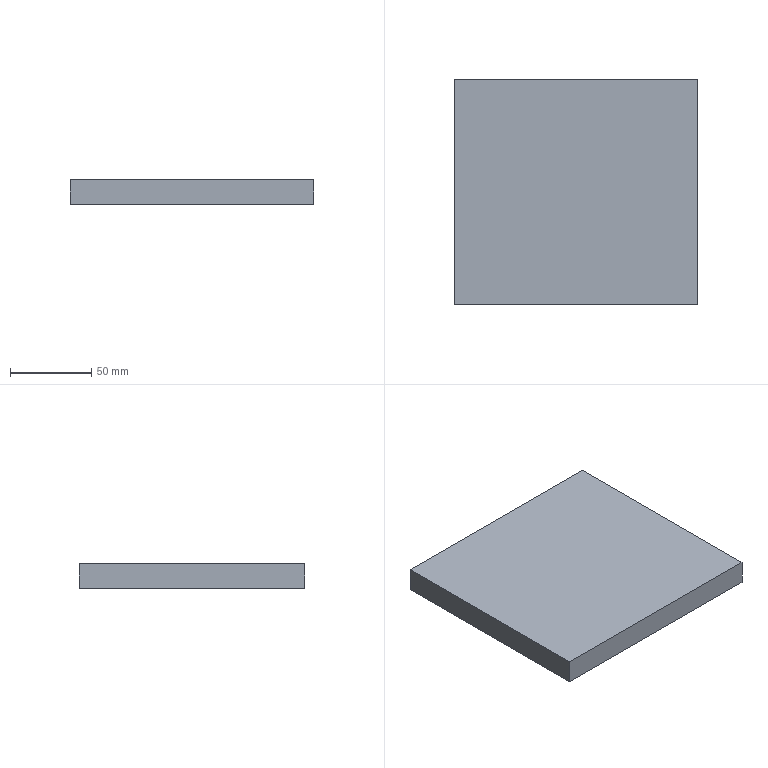Part | STEP file | PN_0004 | 1 solid | 6 faces | box 150 x 139 x 15 mm | volume 312750 mm3 | plane 6
STEP:
#1=CARTESIAN_POINT('',(0.,0.,0.));
#2=DIRECTION('',(0.,0.,1.));
#3=DIRECTION('',(1.,0.,0.));
#4=AXIS2_PLACEMENT_3D('',#1,#2,#3);
#5=CARTESIAN_POINT('',(75.,-69.5,0.));
#6=VERTEX_POINT('',#5);
#7=CARTESIAN_POINT('',(75.,69.5,0.));
#8=VERTEX_POINT('',#7);
#9=CARTESIAN_POINT('',(75.,69.5,0.));
#10=DIRECTION('',(0.,1.,0.));
#11=VECTOR('',#10,1.);
#12=LINE('',#9,#11);
#13=CARTESIAN_POINT('',(75.,69.5,15.));
#14=DIRECTION('',(-1.,0.,0.));
#15=DIRECTION('',(0.,-1.,0.));
#16=AXIS2_PLACEMENT_3D('',#13,#14,#15);
#17=PLANE('',#16);
#18=CARTESIAN_POINT('',(0.,-15.));
#19=DIRECTION('',(-1.,0.));
#20=VECTOR('',#19,1.);
#21=LINE('',#18,#20);
#22=(GEOMETRIC_REPRESENTATION_CONTEXT(2)PARAMETRIC_REPRESENTATION_CONTEXT()REPRESENTATION_CONTEXT('',''));
#23=DEFINITIONAL_REPRESENTATION('',(#21),#22);
#24=PCURVE('',#17,#23);
#25=CARTESIAN_POINT('',(75.,-69.5,0.));
#26=DIRECTION('',(0.,0.,1.));
#27=DIRECTION('',(1.,0.,0.));
#28=AXIS2_PLACEMENT_3D('',#25,#26,#27);
#29=PLANE('',#28);
#30=CARTESIAN_POINT('',(0.,139.));
#31=DIRECTION('',(0.,1.));
#32=VECTOR('',#31,1.);
#33=LINE('',#30,#32);
#34=(GEOMETRIC_REPRESENTATION_CONTEXT(2)PARAMETRIC_REPRESENTATION_CONTEXT()REPRESENTATION_CONTEXT('',''));
#35=DEFINITIONAL_REPRESENTATION('',(#33),#34);
#36=PCURVE('',#29,#35);
#37=SURFACE_CURVE('',#12,(#24,#36),.PCURVE_S1.);
#38=EDGE_CURVE('',#6,#8,#37,.T.);
#39=ORIENTED_EDGE('',*,*,#38,.T.);
#40=CARTESIAN_POINT('',(75.,69.5,15.));
#41=VERTEX_POINT('',#40);
#42=CARTESIAN_POINT('',(75.,69.5,15.));
#43=DIRECTION('',(0.,0.,-1.));
#44=VECTOR('',#43,1.);
#45=LINE('',#42,#44);
#46=CARTESIAN_POINT('',(0.,0.));
#47=DIRECTION('',(0.,-1.));
#48=VECTOR('',#47,1.);
#49=LINE('',#46,#48);
#50=(GEOMETRIC_REPRESENTATION_CONTEXT(2)PARAMETRIC_REPRESENTATION_CONTEXT()REPRESENTATION_CONTEXT('',''));
#51=DEFINITIONAL_REPRESENTATION('',(#49),#50);
#52=PCURVE('',#17,#51);
#53=CARTESIAN_POINT('',(-75.,69.5,15.));
#54=DIRECTION('',(0.,-1.,0.));
#55=DIRECTION('',(0.,0.,-1.));
#56=AXIS2_PLACEMENT_3D('',#53,#54,#55);
#57=PLANE('',#56);
#58=CARTESIAN_POINT('',(0.,150.));
#59=DIRECTION('',(1.,0.));
#60=VECTOR('',#59,1.);
#61=LINE('',#58,#60);
#62=(GEOMETRIC_REPRESENTATION_CONTEXT(2)PARAMETRIC_REPRESENTATION_CONTEXT()REPRESENTATION_CONTEXT('',''));
#63=DEFINITIONAL_REPRESENTATION('',(#61),#62);
#64=PCURVE('',#57,#63);
#65=SURFACE_CURVE('',#45,(#52,#64),.PCURVE_S1.);
#66=EDGE_CURVE('',#41,#8,#65,.T.);
#67=ORIENTED_EDGE('',*,*,#66,.F.);
#68=CARTESIAN_POINT('',(75.,-69.5,15.));
#69=VERTEX_POINT('',#68);
#70=CARTESIAN_POINT('',(75.,69.5,15.));
#71=DIRECTION('',(0.,1.,0.));
#72=VECTOR('',#71,1.);
#73=LINE('',#70,#72);
#74=CARTESIAN_POINT('',(0.,0.));
#75=DIRECTION('',(-1.,0.));
#76=VECTOR('',#75,1.);
#77=LINE('',#74,#76);
#78=(GEOMETRIC_REPRESENTATION_CONTEXT(2)PARAMETRIC_REPRESENTATION_CONTEXT()REPRESENTATION_CONTEXT('',''));
#79=DEFINITIONAL_REPRESENTATION('',(#77),#78);
#80=PCURVE('',#17,#79);
#81=CARTESIAN_POINT('',(75.,-69.5,15.));
#82=DIRECTION('',(0.,0.,1.));
#83=DIRECTION('',(1.,0.,0.));
#84=AXIS2_PLACEMENT_3D('',#81,#82,#83);
#85=PLANE('',#84);
#86=CARTESIAN_POINT('',(0.,139.));
#87=DIRECTION('',(0.,1.));
#88=VECTOR('',#87,1.);
#89=LINE('',#86,#88);
#90=(GEOMETRIC_REPRESENTATION_CONTEXT(2)PARAMETRIC_REPRESENTATION_CONTEXT()REPRESENTATION_CONTEXT('',''));
#91=DEFINITIONAL_REPRESENTATION('',(#89),#90);
#92=PCURVE('',#85,#91);
#93=SURFACE_CURVE('',#73,(#80,#92),.PCURVE_S1.);
#94=EDGE_CURVE('',#69,#41,#93,.T.);
#95=ORIENTED_EDGE('',*,*,#94,.F.);
#96=CARTESIAN_POINT('',(75.,-69.5,15.));
#97=DIRECTION('',(0.,0.,-1.));
#98=VECTOR('',#97,1.);
#99=LINE('',#96,#98);
#100=CARTESIAN_POINT('',(139.,0.));
#101=DIRECTION('',(0.,-1.));
#102=VECTOR('',#101,1.);
#103=LINE('',#100,#102);
#104=(GEOMETRIC_REPRESENTATION_CONTEXT(2)PARAMETRIC_REPRESENTATION_CONTEXT()REPRESENTATION_CONTEXT('',''));
#105=DEFINITIONAL_REPRESENTATION('',(#103),#104);
#106=PCURVE('',#17,#105);
#107=CARTESIAN_POINT('',(-75.,-69.5,15.));
#108=DIRECTION('',(0.,1.,0.));
#109=DIRECTION('',(0.,0.,1.));
#110=AXIS2_PLACEMENT_3D('',#107,#108,#109);
#111=PLANE('',#110);
#112=CARTESIAN_POINT('',(0.,150.));
#113=DIRECTION('',(-1.,0.));
#114=VECTOR('',#113,1.);
#115=LINE('',#112,#114);
#116=(GEOMETRIC_REPRESENTATION_CONTEXT(2)PARAMETRIC_REPRESENTATION_CONTEXT()REPRESENTATION_CONTEXT('',''));
#117=DEFINITIONAL_REPRESENTATION('',(#115),#116);
#118=PCURVE('',#111,#117);
#119=SURFACE_CURVE('',#99,(#106,#118),.PCURVE_S1.);
#120=EDGE_CURVE('',#69,#6,#119,.T.);
#121=ORIENTED_EDGE('',*,*,#120,.T.);
#122=EDGE_LOOP('',(#39,#67,#95,#121));
#123=FACE_BOUND('',#122,.T.);
#124=ADVANCED_FACE('',(#123),#17,.F.);
#125=CARTESIAN_POINT('',(-75.,69.5,0.));
#126=VERTEX_POINT('',#125);
#127=CARTESIAN_POINT('',(-75.,69.5,0.));
#128=DIRECTION('',(-1.,0.,0.));
#129=VECTOR('',#128,1.);
#130=LINE('',#127,#129);
#131=CARTESIAN_POINT('',(15.,0.));
#132=DIRECTION('',(0.,-1.));
#133=VECTOR('',#132,1.);
#134=LINE('',#131,#133);
#135=(GEOMETRIC_REPRESENTATION_CONTEXT(2)PARAMETRIC_REPRESENTATION_CONTEXT()REPRESENTATION_CONTEXT('',''));
#136=DEFINITIONAL_REPRESENTATION('',(#134),#135);
#137=PCURVE('',#57,#136);
#138=CARTESIAN_POINT('',(-150.,139.));
#139=DIRECTION('',(-1.,0.));
#140=VECTOR('',#139,1.);
#141=LINE('',#138,#140);
#142=(GEOMETRIC_REPRESENTATION_CONTEXT(2)PARAMETRIC_REPRESENTATION_CONTEXT()REPRESENTATION_CONTEXT('',''));
#143=DEFINITIONAL_REPRESENTATION('',(#141),#142);
#144=PCURVE('',#29,#143);
#145=SURFACE_CURVE('',#130,(#137,#144),.PCURVE_S1.);
#146=EDGE_CURVE('',#8,#126,#145,.T.);
#147=ORIENTED_EDGE('',*,*,#146,.T.);
#148=CARTESIAN_POINT('',(-75.,69.5,15.));
#149=VERTEX_POINT('',#148);
#150=CARTESIAN_POINT('',(-75.,69.5,15.));
#151=DIRECTION('',(0.,0.,-1.));
#152=VECTOR('',#151,1.);
#153=LINE('',#150,#152);
#154=CARTESIAN_POINT('',(0.,0.));
#155=DIRECTION('',(1.,0.));
#156=VECTOR('',#155,1.);
#157=LINE('',#154,#156);
#158=(GEOMETRIC_REPRESENTATION_CONTEXT(2)PARAMETRIC_REPRESENTATION_CONTEXT()REPRESENTATION_CONTEXT('',''));
#159=DEFINITIONAL_REPRESENTATION('',(#157),#158);
#160=PCURVE('',#57,#159);
#161=CARTESIAN_POINT('',(-75.,69.5,15.));
#162=DIRECTION('',(1.,0.,0.));
#163=DIRECTION('',(0.,1.,0.));
#164=AXIS2_PLACEMENT_3D('',#161,#162,#163);
#165=PLANE('',#164);
#166=CARTESIAN_POINT('',(0.,0.));
#167=DIRECTION('',(0.,-1.));
#168=VECTOR('',#167,1.);
#169=LINE('',#166,#168);
#170=(GEOMETRIC_REPRESENTATION_CONTEXT(2)PARAMETRIC_REPRESENTATION_CONTEXT()REPRESENTATION_CONTEXT('',''));
#171=DEFINITIONAL_REPRESENTATION('',(#169),#170);
#172=PCURVE('',#165,#171);
#173=SURFACE_CURVE('',#153,(#160,#172),.PCURVE_S1.);
#174=EDGE_CURVE('',#149,#126,#173,.T.);
#175=ORIENTED_EDGE('',*,*,#174,.F.);
#176=CARTESIAN_POINT('',(-75.,69.5,15.));
#177=DIRECTION('',(-1.,0.,0.));
#178=VECTOR('',#177,1.);
#179=LINE('',#176,#178);
#180=CARTESIAN_POINT('',(0.,0.));
#181=DIRECTION('',(0.,-1.));
#182=VECTOR('',#181,1.);
#183=LINE('',#180,#182);
#184=(GEOMETRIC_REPRESENTATION_CONTEXT(2)PARAMETRIC_REPRESENTATION_CONTEXT()REPRESENTATION_CONTEXT('',''));
#185=DEFINITIONAL_REPRESENTATION('',(#183),#184);
#186=PCURVE('',#57,#185);
#187=CARTESIAN_POINT('',(-150.,139.));
#188=DIRECTION('',(-1.,0.));
#189=VECTOR('',#188,1.);
#190=LINE('',#187,#189);
#191=(GEOMETRIC_REPRESENTATION_CONTEXT(2)PARAMETRIC_REPRESENTATION_CONTEXT()REPRESENTATION_CONTEXT('',''));
#192=DEFINITIONAL_REPRESENTATION('',(#190),#191);
#193=PCURVE('',#85,#192);
#194=SURFACE_CURVE('',#179,(#186,#193),.PCURVE_S1.);
#195=EDGE_CURVE('',#41,#149,#194,.T.);
#196=ORIENTED_EDGE('',*,*,#195,.F.);
#197=ORIENTED_EDGE('',*,*,#66,.T.);
#198=EDGE_LOOP('',(#147,#175,#196,#197));
#199=FACE_BOUND('',#198,.T.);
#200=ADVANCED_FACE('',(#199),#57,.F.);
#201=CARTESIAN_POINT('',(-75.,-69.5,0.));
#202=VERTEX_POINT('',#201);
#203=CARTESIAN_POINT('',(-75.,69.5,0.));
#204=DIRECTION('',(0.,-1.,0.));
#205=VECTOR('',#204,1.);
#206=LINE('',#203,#205);
#207=CARTESIAN_POINT('',(0.,-15.));
#208=DIRECTION('',(-1.,0.));
#209=VECTOR('',#208,1.);
#210=LINE('',#207,#209);
#211=(GEOMETRIC_REPRESENTATION_CONTEXT(2)PARAMETRIC_REPRESENTATION_CONTEXT()REPRESENTATION_CONTEXT('',''));
#212=DEFINITIONAL_REPRESENTATION('',(#210),#211);
#213=PCURVE('',#165,#212);
#214=CARTESIAN_POINT('',(-150.,139.));
#215=DIRECTION('',(0.,-1.));
#216=VECTOR('',#215,1.);
#217=LINE('',#214,#216);
#218=(GEOMETRIC_REPRESENTATION_CONTEXT(2)PARAMETRIC_REPRESENTATION_CONTEXT()REPRESENTATION_CONTEXT('',''));
#219=DEFINITIONAL_REPRESENTATION('',(#217),#218);
#220=PCURVE('',#29,#219);
#221=SURFACE_CURVE('',#206,(#213,#220),.PCURVE_S1.);
#222=EDGE_CURVE('',#126,#202,#221,.T.);
#223=ORIENTED_EDGE('',*,*,#222,.T.);
#224=CARTESIAN_POINT('',(-75.,-69.5,15.));
#225=VERTEX_POINT('',#224);
#226=CARTESIAN_POINT('',(-75.,-69.5,15.));
#227=DIRECTION('',(0.,0.,-1.));
#228=VECTOR('',#227,1.);
#229=LINE('',#226,#228);
#230=CARTESIAN_POINT('',(-139.,0.));
#231=DIRECTION('',(0.,-1.));
#232=VECTOR('',#231,1.);
#233=LINE('',#230,#232);
#234=(GEOMETRIC_REPRESENTATION_CONTEXT(2)PARAMETRIC_REPRESENTATION_CONTEXT()REPRESENTATION_CONTEXT('',''));
#235=DEFINITIONAL_REPRESENTATION('',(#233),#234);
#236=PCURVE('',#165,#235);
#237=CARTESIAN_POINT('',(0.,0.));
#238=DIRECTION('',(-1.,0.));
#239=VECTOR('',#238,1.);
#240=LINE('',#237,#239);
#241=(GEOMETRIC_REPRESENTATION_CONTEXT(2)PARAMETRIC_REPRESENTATION_CONTEXT()REPRESENTATION_CONTEXT('',''));
#242=DEFINITIONAL_REPRESENTATION('',(#240),#241);
#243=PCURVE('',#111,#242);
#244=SURFACE_CURVE('',#229,(#236,#243),.PCURVE_S1.);
#245=EDGE_CURVE('',#225,#202,#244,.T.);
#246=ORIENTED_EDGE('',*,*,#245,.F.);
#247=CARTESIAN_POINT('',(-75.,69.5,15.));
#248=DIRECTION('',(0.,-1.,0.));
#249=VECTOR('',#248,1.);
#250=LINE('',#247,#249);
#251=CARTESIAN_POINT('',(0.,0.));
#252=DIRECTION('',(-1.,0.));
#253=VECTOR('',#252,1.);
#254=LINE('',#251,#253);
#255=(GEOMETRIC_REPRESENTATION_CONTEXT(2)PARAMETRIC_REPRESENTATION_CONTEXT()REPRESENTATION_CONTEXT('',''));
#256=DEFINITIONAL_REPRESENTATION('',(#254),#255);
#257=PCURVE('',#165,#256);
#258=CARTESIAN_POINT('',(-150.,139.));
#259=DIRECTION('',(0.,-1.));
#260=VECTOR('',#259,1.);
#261=LINE('',#258,#260);
#262=(GEOMETRIC_REPRESENTATION_CONTEXT(2)PARAMETRIC_REPRESENTATION_CONTEXT()REPRESENTATION_CONTEXT('',''));
#263=DEFINITIONAL_REPRESENTATION('',(#261),#262);
#264=PCURVE('',#85,#263);
#265=SURFACE_CURVE('',#250,(#257,#264),.PCURVE_S1.);
#266=EDGE_CURVE('',#149,#225,#265,.T.);
#267=ORIENTED_EDGE('',*,*,#266,.F.);
#268=ORIENTED_EDGE('',*,*,#174,.T.);
#269=EDGE_LOOP('',(#223,#246,#267,#268));
#270=FACE_BOUND('',#269,.T.);
#271=ADVANCED_FACE('',(#270),#165,.F.);
#272=CARTESIAN_POINT('',(-75.,-69.5,0.));
#273=DIRECTION('',(1.,0.,0.));
#274=VECTOR('',#273,1.);
#275=LINE('',#272,#274);
#276=CARTESIAN_POINT('',(-15.,0.));
#277=DIRECTION('',(0.,1.));
#278=VECTOR('',#277,1.);
#279=LINE('',#276,#278);
#280=(GEOMETRIC_REPRESENTATION_CONTEXT(2)PARAMETRIC_REPRESENTATION_CONTEXT()REPRESENTATION_CONTEXT('',''));
#281=DEFINITIONAL_REPRESENTATION('',(#279),#280);
#282=PCURVE('',#111,#281);
#283=CARTESIAN_POINT('',(-150.,0.));
#284=DIRECTION('',(1.,0.));
#285=VECTOR('',#284,1.);
#286=LINE('',#283,#285);
#287=(GEOMETRIC_REPRESENTATION_CONTEXT(2)PARAMETRIC_REPRESENTATION_CONTEXT()REPRESENTATION_CONTEXT('',''));
#288=DEFINITIONAL_REPRESENTATION('',(#286),#287);
#289=PCURVE('',#29,#288);
#290=SURFACE_CURVE('',#275,(#282,#289),.PCURVE_S1.);
#291=EDGE_CURVE('',#202,#6,#290,.T.);
#292=ORIENTED_EDGE('',*,*,#291,.T.);
#293=ORIENTED_EDGE('',*,*,#120,.F.);
#294=CARTESIAN_POINT('',(-75.,-69.5,15.));
#295=DIRECTION('',(1.,0.,0.));
#296=VECTOR('',#295,1.);
#297=LINE('',#294,#296);
#298=CARTESIAN_POINT('',(0.,0.));
#299=DIRECTION('',(0.,1.));
#300=VECTOR('',#299,1.);
#301=LINE('',#298,#300);
#302=(GEOMETRIC_REPRESENTATION_CONTEXT(2)PARAMETRIC_REPRESENTATION_CONTEXT()REPRESENTATION_CONTEXT('',''));
#303=DEFINITIONAL_REPRESENTATION('',(#301),#302);
#304=PCURVE('',#111,#303);
#305=CARTESIAN_POINT('',(-150.,0.));
#306=DIRECTION('',(1.,0.));
#307=VECTOR('',#306,1.);
#308=LINE('',#305,#307);
#309=(GEOMETRIC_REPRESENTATION_CONTEXT(2)PARAMETRIC_REPRESENTATION_CONTEXT()REPRESENTATION_CONTEXT('',''));
#310=DEFINITIONAL_REPRESENTATION('',(#308),#309);
#311=PCURVE('',#85,#310);
#312=SURFACE_CURVE('',#297,(#304,#311),.PCURVE_S1.);
#313=EDGE_CURVE('',#225,#69,#312,.T.);
#314=ORIENTED_EDGE('',*,*,#313,.F.);
#315=ORIENTED_EDGE('',*,*,#245,.T.);
#316=EDGE_LOOP('',(#292,#293,#314,#315));
#317=FACE_BOUND('',#316,.T.);
#318=ADVANCED_FACE('',(#317),#111,.F.);
#319=ORIENTED_EDGE('',*,*,#94,.T.);
#320=ORIENTED_EDGE('',*,*,#195,.T.);
#321=ORIENTED_EDGE('',*,*,#266,.T.);
#322=ORIENTED_EDGE('',*,*,#313,.T.);
#323=EDGE_LOOP('',(#319,#320,#321,#322));
#324=FACE_BOUND('',#323,.T.);
#325=ADVANCED_FACE('',(#324),#85,.T.);
#326=ORIENTED_EDGE('',*,*,#38,.F.);
#327=ORIENTED_EDGE('',*,*,#291,.F.);
#328=ORIENTED_EDGE('',*,*,#222,.F.);
#329=ORIENTED_EDGE('',*,*,#146,.F.);
#330=EDGE_LOOP('',(#326,#327,#328,#329));
#331=FACE_BOUND('',#330,.T.);
#332=ADVANCED_FACE('',(#331),#29,.F.);
#333=CLOSED_SHELL('',(#124,#200,#271,#318,#325,#332));
#334=MANIFOLD_SOLID_BREP('',#333);
#335=(LENGTH_UNIT()NAMED_UNIT(*)SI_UNIT(.MILLI.,.METRE.));
#336=UNCERTAINTY_MEASURE_WITH_UNIT(LENGTH_MEASURE(0.0000001),#335,'','');
#337=(NAMED_UNIT(*)PLANE_ANGLE_UNIT()SI_UNIT($,.RADIAN.));
#338=(NAMED_UNIT(*)SI_UNIT($,.STERADIAN.)SOLID_ANGLE_UNIT());
#339=(GEOMETRIC_REPRESENTATION_CONTEXT(3)GLOBAL_UNCERTAINTY_ASSIGNED_CONTEXT((#336))GLOBAL_UNIT_ASSIGNED_CONTEXT((#335,#337,#338))REPRESENTATION_CONTEXT('',''));
#340=ADVANCED_BREP_SHAPE_REPRESENTATION('',(#4,#334),#339);